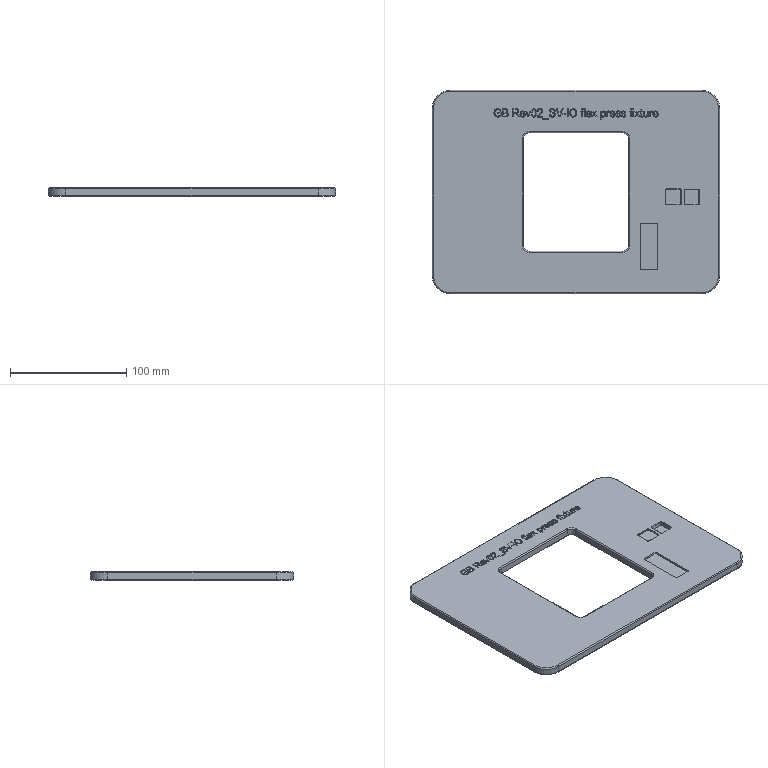CAM job | NX | 3-axis milling | part box 247.208 x 175.016 x 7.2 mm | stock box 252.208 x 180.016 x 8 mm
Tools:
number,name,description,diameter,corner_radius,flute_length,length,flutes
3,D3,平底铣刀-粗,3.0,0.0,20.0,75.0,2
6,D6,平底铣刀-粗,6.0,0.0,25.0,75.0,2
9,D10,平底铣刀-粗,10.0,0.0,35.0,75.0,2
17,D1.5-J,平底铣刀-粗,1.5,0.0,50.0,75.0,2
11,D3-J,平底铣刀-精,3.0,0.0,50.0,75.0,2
7,D6-J,平底铣刀-精,6.0,0.0,25.0,75.0,2
18,D4R0.5,圆鼻刀-粗,4.0,0.5,50.0,75.0,2
1,D80R0.8飞刀,圆鼻刀-粗,80.0,0.8,50.0,75.0,2
1,D80R0.8飞刀-J,圆鼻刀-精,80.0,0.8,50.0,75.0,2
2,D6倒角刀,倒角刀,6.0,0.0,3.0,25.0,2
Operations:
program,operation,operation_type,tool,method,geometry_group,spindle_rpm,surface_speed,feed_per_tooth,feed_cut,feed_plunge,cut_length_mm,path_length_mm,cut_time_min,machine_time_min
B,底壁铣分层开粗-中_COPY,VolumeBased25DMillingOperation,D6,分层开粗-切深K-步距G,W-B,8000.0,150.796,0.125,2000.0,100.0,3857.251,4426.094,1.929,1.986
B,平面去毛刺6X45L_COPY,SurfaceContour,D6倒角刀,爬面_倒角-切深0-步距G,W-B,6500.0,122.519,0.1154,1500.0,100.0,266.212,752.56,0.1775,0.2261
B,等高螺旋爬面_COPY_COPY,ZLevelMilling,D4R0.5,等高爬面-切深K-步距G,W-B,7000.0,87.965,0.3571,5000.0,100.0,28739.179,29020.175,5.748,5.776
B,底壁铣精光底面-中_COPY,VolumeBased25DMillingOperation,D6-J,精光步距切深关,W-B,8000.0,150.792,0.0625,1000.0,100.0,432.534,860.999,0.4325,0.4754
B,底壁铣精光侧面-中-选底面_COPY,VolumeBased25DMillingOperation,D6-J,侧刃精光-切深K-步距G,W-B,8000.0,150.792,0.0625,1000.0,100.0,228.195,674.51,0.2282,0.2728
A,底壁铣飞面开粗_COPY,VolumeBased25DMillingOperation,D80R0.8飞刀,分层开粗-切深K-步距G,W-A,2800.0,703.696,0.5357,3000.0,100.0,2232.65,2639.277,0.7442,0.7849
A,底壁铣飞面精光_COPY,VolumeBased25DMillingOperation,D80R0.8飞刀-J,侧刃精光-切深K-步距G,W-A,4000.0,1005.28,0.125,1000.0,100.0,1115.541,1151.541,1.115,1.119
A,底壁粗_1,VolumeBased25DMillingOperation,D6,METHOD,W-A,6000.0,113.0,0.2083,3500.0,100.0,705.526,776.391,0.2016,0.2087
A,底壁粗_2,VolumeBased25DMillingOperation,D3,METHOD,W-A,6000.0,56.549,0.0833,1000.0,100.0,602.707,664.746,0.6027,0.6089
A,底壁粗_3,VolumeBased25DMillingOperation,D3,METHOD,W-A,6000.0,56.549,0.0833,1000.0,100.0,1707.97,1868.101,1.708,1.724
A,清角D4,ZLevelMilling,D1.5-J,METHOD,W-A,9000.0,42.411,0.0833,1500.0,80.0,793.443,1588.359,0.5464,0.6259
A,清角D4_COPY,ZLevelMilling,D1.5-J,METHOD,W-A,9000.0,42.411,0.0833,1500.0,80.0,1379.328,1545.257,0.9219,0.9385
A,外形粗_2,VolumeBased25DMillingOperation,D10,METHOD,W-A,6000.0,188.0,0.25,4000.0,80.0,19119.288,19310.871,4.78,4.799
A,底精_1,VolumeBased25DMillingOperation,D3-J,METHOD,W-A,6000.0,113.0,0.2083,1200.0,100.0,338.931,380.331,0.2824,0.2866
A,底精_2,VolumeBased25DMillingOperation,D3-J,METHOD,W-A,6000.0,113.0,0.0667,800.0,100.0,112.736,152.976,0.1409,0.1449
A,底精_3,VolumeBased25DMillingOperation,D3-J,METHOD,W-A,6000.0,113.0,0.0667,800.0,100.0,106.151,151.434,0.1327,0.1372
A,等高螺旋爬面_COPY,ZLevelMilling,D4R0.5,等高爬面-切深K-步距G,W-A,7000.0,87.965,0.3571,5000.0,100.0,28739.178,28900.178,5.748,5.764
A,仅选体,SurfaceContour,D6倒角刀,METHOD,W-A,6000.0,113.0,0.125,1200.0,100.0,108.745,144.546,0.0906,0.0942
A,底壁铣倒角_COPY,VolumeBased25DMillingOperation,D6倒角刀,爬面_倒角-切深0-步距G,W-A,6500.0,122.519,0.1154,1500.0,100.0,105.182,198.754,0.0701,0.0795
A,底侧精_4,VolumeBased25DMillingOperation,D3-J,METHOD,W-A,6000.0,113.0,0.0667,800.0,100.0,45.12,86.35,0.0564,0.0605
A,底侧精_5,VolumeBased25DMillingOperation,D3-J,METHOD,W-A,6000.0,113.0,0.0667,800.0,100.0,42.925,89.198,0.0537,0.0583
A,底侧精_3,VolumeBased25DMillingOperation,D3-J,METHOD,W-A,6000.0,113.0,0.2083,1200.0,100.0,102.842,145.232,0.0857,0.0899
A,外形半精_2,VolumeBased25DMillingOperation,D6-J,METHOD,W-A,6000.0,113.0,0.0833,1000.0,100.0,1205.995,1391.378,1.206,1.224
A,外形精_2,VolumeBased25DMillingOperation,D6-J,METHOD,W-A,6000.0,113.0,0.0833,1000.0,100.0,1205.595,1392.039,1.206,1.224